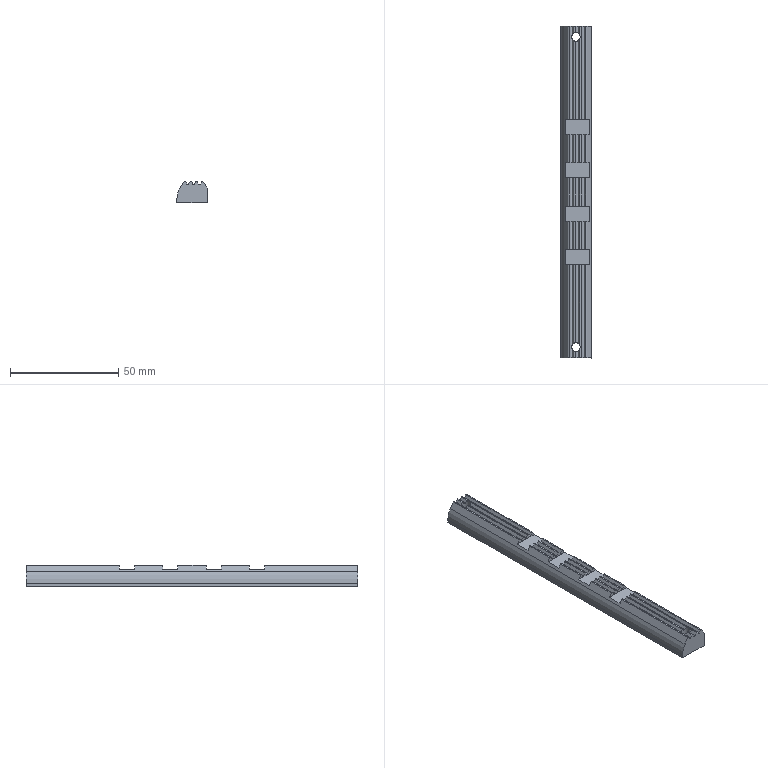Part | STEP file | 1 solid | 97 faces | box 14 x 153 x 10 mm | volume 17764 mm3 | plane 55 | cylinder 42 | commonest cylinder face diameters 0.6 x22 0.8 x17 4 x2 20 x1